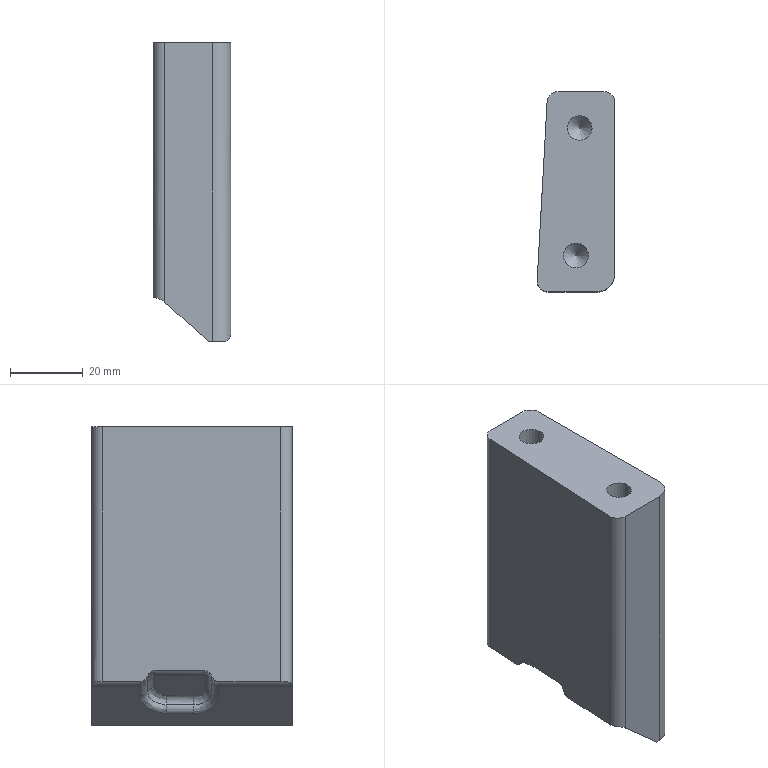Part | NX | features solid 2 | 1 solid | 43 faces | box 21.35 x 55 x 82 mm | volume 80871 mm3 | cylinder 18 | spline 14 | plane 9 | cone 2 | commonest cylinder face diameters 4 x9 10 x4 6 x3 6.8 x2